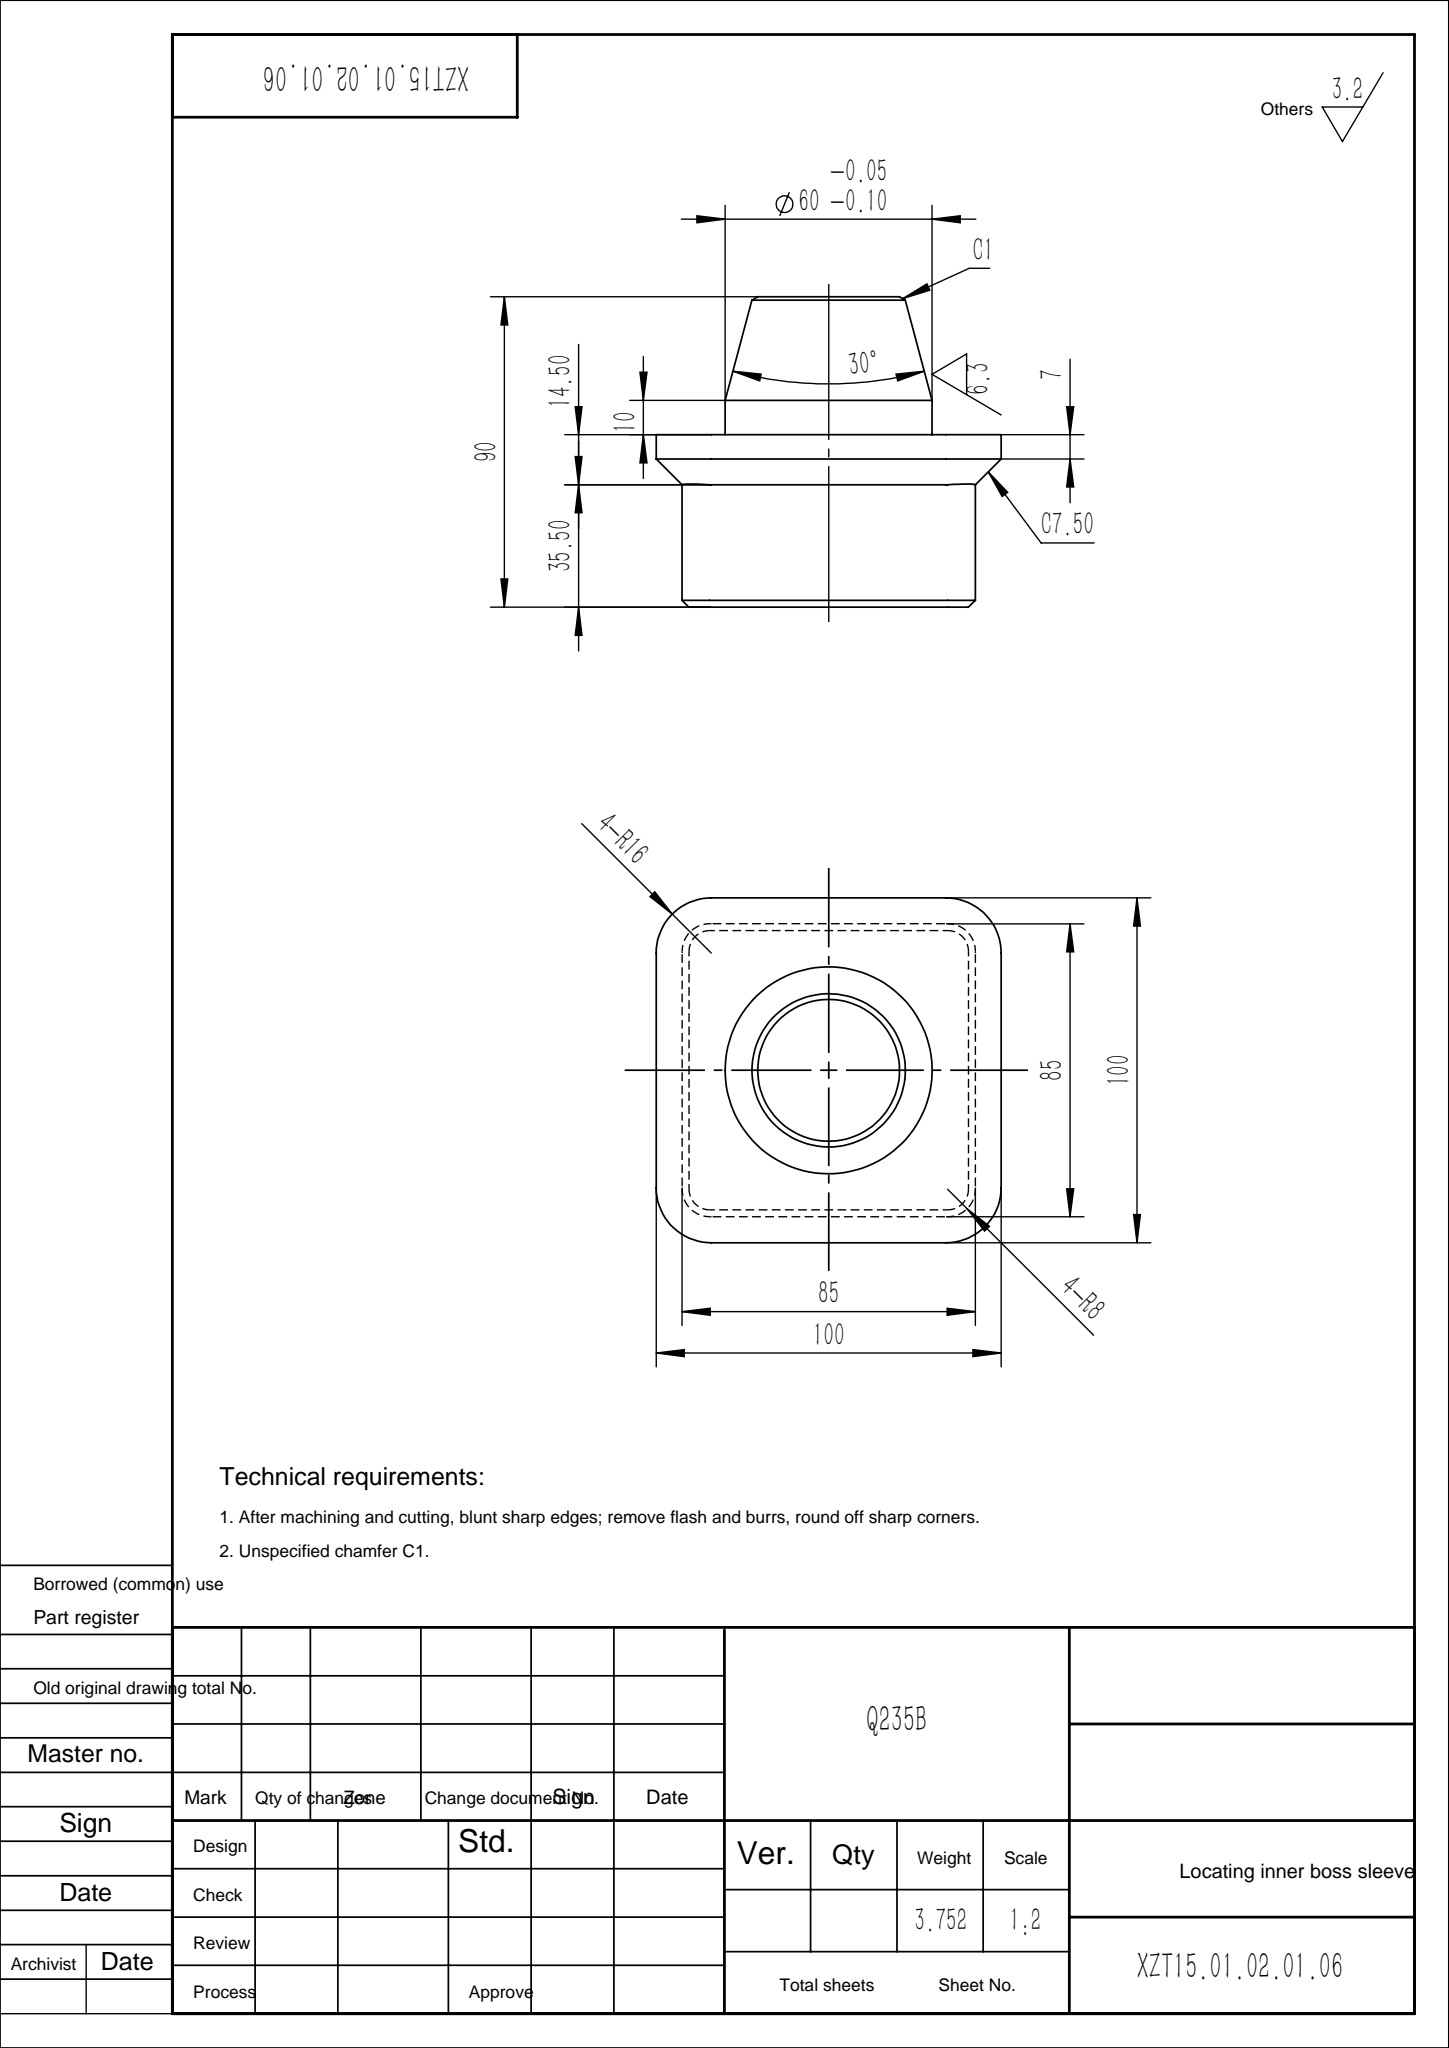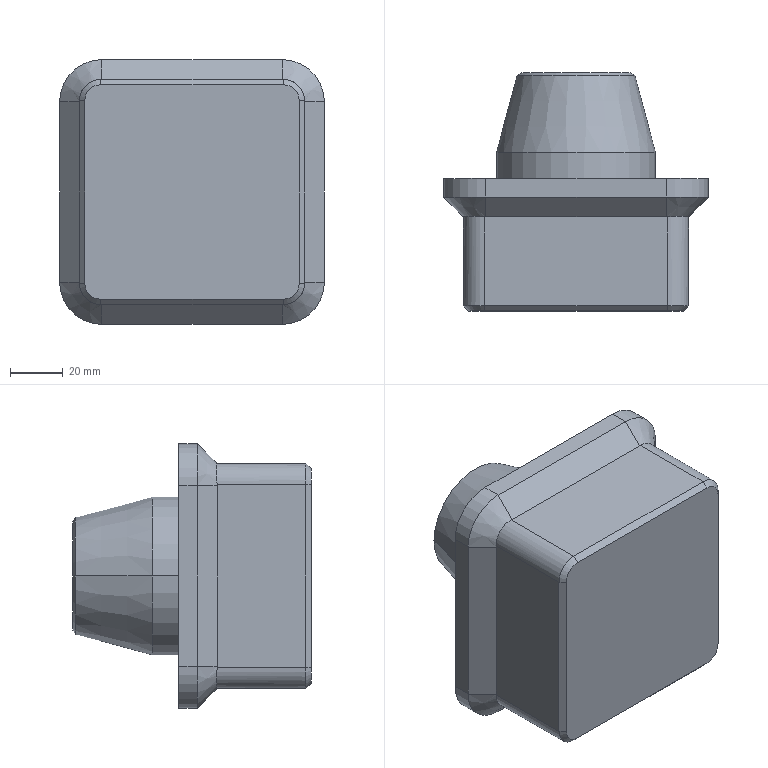Part | SolidWorks | features Chamfer 3, ICE 2, Revolution 1 | 1 solid | 41 faces | box 100 x 90 x 100 mm | volume 477978 mm3 | plane 19 | cone 12 | cylinder 10 | commonest cylinder face diameters 16 x4 32 x4 60 x2